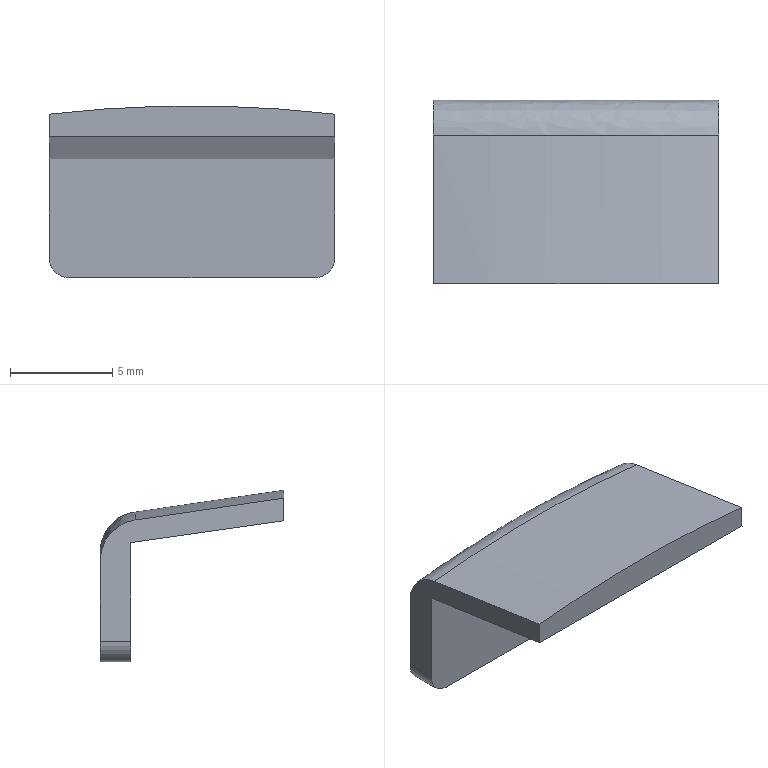Part | STEP file | ZXW735-L-95-05 | 1 solid | 15 faces | box 14 x 9 x 8.417 mm | volume 278.257 mm3 | plane 10 | cylinder 3 | other 1 | spline 1 | commonest cylinder face diameters 2 x2 61.422 x1
STEP:
#1=CARTESIAN_POINT('',(0.,0.,0.));
#2=DIRECTION('',(0.,0.,1.));
#3=DIRECTION('',(1.,0.,0.));
#4=AXIS2_PLACEMENT_3D('',#1,#2,#3);
#5=CARTESIAN_POINT('',(-23.763,12.127,8.554));
#6=VERTEX_POINT('',#5);
#7=CARTESIAN_POINT('',(-37.763,12.127,8.554));
#8=VERTEX_POINT('',#7);
#9=CARTESIAN_POINT('',(-24.693,12.127,8.661));
#10=CARTESIAN_POINT('',(-26.555,12.127,8.833));
#11=CARTESIAN_POINT('',(-29.36,12.127,8.962));
#12=CARTESIAN_POINT('',(-32.167,12.127,8.962));
#13=CARTESIAN_POINT('',(-34.971,12.127,8.833));
#14=CARTESIAN_POINT('',(-36.833,12.127,8.661));
#15=B_SPLINE_CURVE_WITH_KNOTS('',3,(#5,#9,#10,#11,#12,#13,#14,#7),.UNSPECIFIED.,.F.,.F.,(4,1,1,1,1,4),(0.,0.2,0.4,0.6,0.8,1.),.UNSPECIFIED.);
#16=EDGE_CURVE('',#6,#8,#15,.T.);
#17=ORIENTED_EDGE('',*,*,#16,.F.);
#18=CARTESIAN_POINT('',(-23.763,12.127,7.444));
#19=VERTEX_POINT('',#18);
#20=CARTESIAN_POINT('',(-23.763,12.127,7.444));
#21=DIRECTION('',(0.00001014,0.00001377,1.));
#22=VECTOR('',#21,1.11);
#23=LINE('',#20,#22);
#24=EDGE_CURVE('',#19,#6,#23,.T.);
#25=ORIENTED_EDGE('',*,*,#24,.F.);
#26=CARTESIAN_POINT('',(-37.763,12.127,7.444));
#27=VERTEX_POINT('',#26);
#28=CARTESIAN_POINT('',(-37.763,12.127,7.444));
#29=DIRECTION('',(1.,0.,0.000000407));
#30=VECTOR('',#29,14.);
#31=LINE('',#28,#30);
#32=EDGE_CURVE('',#27,#19,#31,.T.);
#33=ORIENTED_EDGE('',*,*,#32,.F.);
#34=CARTESIAN_POINT('',(-37.763,12.127,7.444));
#35=DIRECTION('',(-0.00001151,0.00000571,1.));
#36=VECTOR('',#35,1.11);
#37=LINE('',#34,#36);
#38=EDGE_CURVE('',#27,#8,#37,.T.);
#39=ORIENTED_EDGE('',*,*,#38,.T.);
#40=EDGE_LOOP('',(#17,#25,#33,#39));
#41=FACE_OUTER_BOUND('',#40,.F.);
#42=CARTESIAN_POINT('',(-37.363,12.127,5.74));
#43=DIRECTION('',(0.,1.,0.));
#44=DIRECTION('',(-1.,0.,-0.000000599));
#45=AXIS2_PLACEMENT_3D('',#42,#43,#44);
#46=PLANE('',#45);
#47=ADVANCED_FACE('',(#41),#46,.F.);
#48=CARTESIAN_POINT('',(-23.763,19.417,7.482));
#49=VERTEX_POINT('',#48);
#50=CARTESIAN_POINT('',(-23.763,19.417,7.482));
#51=DIRECTION('',(-0.000000599,-0.9894,0.1455));
#52=VECTOR('',#51,7.368);
#53=LINE('',#50,#52);
#54=EDGE_CURVE('',#49,#6,#53,.T.);
#55=ORIENTED_EDGE('',*,*,#54,.T.);
#56=ORIENTED_EDGE('',*,*,#16,.T.);
#57=CARTESIAN_POINT('',(-37.763,19.417,7.483));
#58=VERTEX_POINT('',#57);
#59=CARTESIAN_POINT('',(-37.763,12.127,8.554));
#60=DIRECTION('',(-0.000000416,0.9894,-0.1455));
#61=VECTOR('',#60,7.368);
#62=LINE('',#59,#61);
#63=EDGE_CURVE('',#8,#58,#62,.T.);
#64=ORIENTED_EDGE('',*,*,#63,.T.);
#65=CARTESIAN_POINT('',(-30.763,19.417,-53.205));
#66=DIRECTION('',(0.,1.,0.));
#67=DIRECTION('',(-0.1146,0.,0.9934));
#68=AXIS2_PLACEMENT_3D('',#65,#66,#67);
#69=CIRCLE('',#68,61.09);
#70=EDGE_CURVE('',#58,#49,#69,.T.);
#71=ORIENTED_EDGE('',*,*,#70,.T.);
#72=EDGE_LOOP('',(#55,#56,#64,#71));
#73=FACE_OUTER_BOUND('',#72,.F.);
#74=CARTESIAN_POINT('',(-30.763,10.927,-51.957));
#75=DIRECTION('',(0.,1.,0.));
#76=DIRECTION('',(-0.1277,0.,0.9918));
#77=AXIS2_PLACEMENT_3D('',#74,#75,#76);
#78=CIRCLE('',#77,61.09);
#79=TRIMMED_CURVE('',#78,(PARAMETER_VALUE(0.)),(PARAMETER_VALUE(14.671)),.T.,.UNSPECIFIED.);
#80=DIRECTION('',(0.00000009,0.9894,-0.1455));
#81=VECTOR('',#80,1.);
#82=SURFACE_OF_LINEAR_EXTRUSION('',#79,#81);
#83=ADVANCED_FACE('',(#73),#82,.T.);
#84=CARTESIAN_POINT('',(-23.763,21.127,1.54));
#85=VERTEX_POINT('',#84);
#86=CARTESIAN_POINT('',(-23.763,21.127,5.49));
#87=VERTEX_POINT('',#86);
#88=CARTESIAN_POINT('',(-23.763,21.127,1.54));
#89=DIRECTION('',(-0.000000635,0.,1.));
#90=VECTOR('',#89,3.95);
#91=LINE('',#88,#90);
#92=EDGE_CURVE('',#85,#87,#91,.T.);
#93=ORIENTED_EDGE('',*,*,#92,.F.);
#94=CARTESIAN_POINT('',(-23.763,19.627,1.54));
#95=VERTEX_POINT('',#94);
#96=CARTESIAN_POINT('',(-23.763,21.127,1.54));
#97=DIRECTION('',(-0.000000163,-1.,-0.000001718));
#98=VECTOR('',#97,1.5);
#99=LINE('',#96,#98);
#100=EDGE_CURVE('',#85,#95,#99,.T.);
#101=ORIENTED_EDGE('',*,*,#100,.T.);
#102=CARTESIAN_POINT('',(-23.763,19.627,6.374));
#103=VERTEX_POINT('',#102);
#104=CARTESIAN_POINT('',(-23.763,19.627,1.54));
#105=DIRECTION('',(-0.000000525,0.,1.));
#106=VECTOR('',#105,4.834);
#107=LINE('',#104,#106);
#108=EDGE_CURVE('',#95,#103,#107,.T.);
#109=ORIENTED_EDGE('',*,*,#108,.T.);
#110=CARTESIAN_POINT('',(-23.763,12.127,7.444));
#111=DIRECTION('',(0.000000107,0.99,-0.1412));
#112=VECTOR('',#111,7.576);
#113=LINE('',#110,#112);
#114=EDGE_CURVE('',#19,#103,#113,.T.);
#115=ORIENTED_EDGE('',*,*,#114,.F.);
#116=ORIENTED_EDGE('',*,*,#24,.T.);
#117=ORIENTED_EDGE('',*,*,#54,.F.);
#118=CARTESIAN_POINT('',(-23.763,19.417,7.482));
#119=CARTESIAN_POINT('',(-23.763,19.535,7.465));
#120=CARTESIAN_POINT('',(-23.763,19.764,7.41));
#121=CARTESIAN_POINT('',(-23.763,20.093,7.265));
#122=CARTESIAN_POINT('',(-23.763,20.39,7.065));
#123=CARTESIAN_POINT('',(-23.763,20.647,6.816));
#124=CARTESIAN_POINT('',(-23.763,20.856,6.524));
#125=CARTESIAN_POINT('',(-23.763,21.01,6.199));
#126=CARTESIAN_POINT('',(-23.763,21.106,5.851));
#127=CARTESIAN_POINT('',(-23.763,21.127,5.612));
#128=CARTESIAN_POINT('',(-23.763,21.127,5.49));
#129=B_SPLINE_CURVE_WITH_KNOTS('',3,(#118,#119,#120,#121,#122,#123,#124,#125,#126,#127,#128),.UNSPECIFIED.,.F.,.F.,(4,1,1,1,1,1,1,1,4),(0.,0.125,0.25,0.375,0.5,0.625,0.75,0.875,1.),.UNSPECIFIED.);
#130=EDGE_CURVE('',#49,#87,#129,.T.);
#131=ORIENTED_EDGE('',*,*,#130,.T.);
#132=EDGE_LOOP('',(#93,#101,#109,#115,#116,#117,#131));
#133=FACE_OUTER_BOUND('',#132,.F.);
#134=CARTESIAN_POINT('',(-23.763,27.279,-9.26));
#135=DIRECTION('',(1.,0.,0.000000621));
#136=DIRECTION('',(-0.000000621,0.,1.));
#137=AXIS2_PLACEMENT_3D('',#134,#135,#136);
#138=PLANE('',#137);
#139=ADVANCED_FACE('',(#133),#138,.T.);
#140=CARTESIAN_POINT('',(-37.763,21.127,1.54));
#141=VERTEX_POINT('',#140);
#142=CARTESIAN_POINT('',(-37.763,21.127,5.49));
#143=VERTEX_POINT('',#142);
#144=CARTESIAN_POINT('',(-37.763,21.127,1.54));
#145=DIRECTION('',(-0.000000625,0.,1.));
#146=VECTOR('',#145,3.95);
#147=LINE('',#144,#146);
#148=EDGE_CURVE('',#141,#143,#147,.T.);
#149=ORIENTED_EDGE('',*,*,#148,.F.);
#150=CARTESIAN_POINT('',(-36.763,21.127,0.5396));
#151=VERTEX_POINT('',#150);
#152=CARTESIAN_POINT('',(-36.763,21.127,1.54));
#153=DIRECTION('',(0.,1.,0.));
#154=DIRECTION('',(0.0000187,0.,-1.));
#155=AXIS2_PLACEMENT_3D('',#152,#153,#154);
#156=CIRCLE('',#155,1.);
#157=EDGE_CURVE('',#151,#141,#156,.T.);
#158=ORIENTED_EDGE('',*,*,#157,.F.);
#159=CARTESIAN_POINT('',(-24.763,21.127,0.5396));
#160=VERTEX_POINT('',#159);
#161=CARTESIAN_POINT('',(-24.763,21.127,0.5396));
#162=DIRECTION('',(-1.,0.,-0.000000397));
#163=VECTOR('',#162,12.);
#164=LINE('',#161,#163);
#165=EDGE_CURVE('',#160,#151,#164,.T.);
#166=ORIENTED_EDGE('',*,*,#165,.F.);
#167=CARTESIAN_POINT('',(-24.763,21.127,1.54));
#168=DIRECTION('',(0.,1.,0.));
#169=DIRECTION('',(1.,0.,-0.000000136));
#170=AXIS2_PLACEMENT_3D('',#167,#168,#169);
#171=CIRCLE('',#170,1.);
#172=EDGE_CURVE('',#85,#160,#171,.T.);
#173=ORIENTED_EDGE('',*,*,#172,.F.);
#174=ORIENTED_EDGE('',*,*,#92,.T.);
#175=CARTESIAN_POINT('',(-37.763,21.127,5.49));
#176=CARTESIAN_POINT('',(-33.119,21.127,6.042));
#177=CARTESIAN_POINT('',(-28.411,21.127,6.042));
#178=CARTESIAN_POINT('',(-23.763,21.127,5.49));
#179=B_SPLINE_CURVE_WITH_KNOTS('',3,(#175,#176,#177,#178),.UNSPECIFIED.,.F.,.F.,(4,4),(0.,1.),.UNSPECIFIED.);
#180=EDGE_CURVE('',#143,#87,#179,.T.);
#181=ORIENTED_EDGE('',*,*,#180,.F.);
#182=EDGE_LOOP('',(#149,#158,#166,#173,#174,#181));
#183=FACE_OUTER_BOUND('',#182,.F.);
#184=CARTESIAN_POINT('',(-36.62,21.127,5.114));
#185=VERTEX_POINT('',#184);
#186=CARTESIAN_POINT('',(-30.763,21.127,1.576));
#187=VERTEX_POINT('',#186);
#188=CARTESIAN_POINT('',(-36.62,21.127,5.114));
#189=DIRECTION('',(0.856,0.,-0.517));
#190=VECTOR('',#189,6.842);
#191=LINE('',#188,#190);
#192=EDGE_CURVE('',#185,#187,#191,.T.);
#193=ORIENTED_EDGE('',*,*,#192,.F.);
#194=CARTESIAN_POINT('',(-24.898,21.127,5.118));
#195=VERTEX_POINT('',#194);
#196=CARTESIAN_POINT('',(-30.772,21.127,35.262));
#197=DIRECTION('',(0.,1.,0.));
#198=DIRECTION('',(0.1912,0.,-0.9815));
#199=AXIS2_PLACEMENT_3D('',#196,#197,#198);
#200=CIRCLE('',#199,30.711);
#201=EDGE_CURVE('',#195,#185,#200,.T.);
#202=ORIENTED_EDGE('',*,*,#201,.F.);
#203=CARTESIAN_POINT('',(-30.763,21.127,1.576));
#204=DIRECTION('',(0.856,0.,0.517));
#205=VECTOR('',#204,6.852);
#206=LINE('',#203,#205);
#207=EDGE_CURVE('',#187,#195,#206,.T.);
#208=ORIENTED_EDGE('',*,*,#207,.F.);
#209=EDGE_LOOP('',(#193,#202,#208));
#210=FACE_BOUND('',#209,.F.);
#211=CARTESIAN_POINT('',(-38.363,21.127,5.74));
#212=DIRECTION('',(0.,1.,0.));
#213=DIRECTION('',(-1.,0.,-0.000000599));
#214=AXIS2_PLACEMENT_3D('',#211,#212,#213);
#215=PLANE('',#214);
#216=ADVANCED_FACE('',(#183,#210),#215,.T.);
#217=CARTESIAN_POINT('',(-30.763,20.877,1.576));
#218=VERTEX_POINT('',#217);
#219=CARTESIAN_POINT('',(-30.763,21.127,1.576));
#220=DIRECTION('',(0.,-1.,0.));
#221=VECTOR('',#220,0.25);
#222=LINE('',#219,#221);
#223=EDGE_CURVE('',#187,#218,#222,.T.);
#224=ORIENTED_EDGE('',*,*,#223,.T.);
#225=CARTESIAN_POINT('',(-36.62,20.877,5.114));
#226=VERTEX_POINT('',#225);
#227=CARTESIAN_POINT('',(-30.763,20.877,1.576));
#228=DIRECTION('',(-0.856,0.,0.517));
#229=VECTOR('',#228,6.842);
#230=LINE('',#227,#229);
#231=EDGE_CURVE('',#218,#226,#230,.T.);
#232=ORIENTED_EDGE('',*,*,#231,.T.);
#233=CARTESIAN_POINT('',(-36.62,20.877,5.114));
#234=DIRECTION('',(0.,1.,0.));
#235=VECTOR('',#234,0.25);
#236=LINE('',#233,#235);
#237=EDGE_CURVE('',#226,#185,#236,.T.);
#238=ORIENTED_EDGE('',*,*,#237,.T.);
#239=ORIENTED_EDGE('',*,*,#192,.T.);
#240=EDGE_LOOP('',(#224,#232,#238,#239));
#241=FACE_OUTER_BOUND('',#240,.F.);
#242=CARTESIAN_POINT('',(-36.731,20.627,5.181));
#243=DIRECTION('',(0.517,0.,0.856));
#244=DIRECTION('',(-0.856,0.,0.517));
#245=AXIS2_PLACEMENT_3D('',#242,#243,#244);
#246=PLANE('',#245);
#247=ADVANCED_FACE('',(#241),#246,.T.);
#248=CARTESIAN_POINT('',(-24.898,20.877,5.118));
#249=VERTEX_POINT('',#248);
#250=CARTESIAN_POINT('',(-24.898,21.127,5.118));
#251=DIRECTION('',(0.,-1.,0.));
#252=VECTOR('',#251,0.25);
#253=LINE('',#250,#252);
#254=EDGE_CURVE('',#195,#249,#253,.T.);
#255=ORIENTED_EDGE('',*,*,#254,.T.);
#256=CARTESIAN_POINT('',(-24.898,20.877,5.118));
#257=DIRECTION('',(-0.856,0.,-0.517));
#258=VECTOR('',#257,6.852);
#259=LINE('',#256,#258);
#260=EDGE_CURVE('',#249,#218,#259,.T.);
#261=ORIENTED_EDGE('',*,*,#260,.T.);
#262=ORIENTED_EDGE('',*,*,#223,.F.);
#263=ORIENTED_EDGE('',*,*,#207,.T.);
#264=EDGE_LOOP('',(#255,#261,#262,#263));
#265=FACE_OUTER_BOUND('',#264,.F.);
#266=CARTESIAN_POINT('',(-30.626,20.627,1.659));
#267=DIRECTION('',(-0.517,0.,0.856));
#268=DIRECTION('',(-0.856,0.,-0.517));
#269=AXIS2_PLACEMENT_3D('',#266,#267,#268);
#270=PLANE('',#269);
#271=ADVANCED_FACE('',(#265),#270,.T.);
#272=ORIENTED_EDGE('',*,*,#237,.F.);
#273=CARTESIAN_POINT('',(-30.772,20.877,35.262));
#274=DIRECTION('',(0.,-1.,0.));
#275=DIRECTION('',(-0.1904,0.,-0.9817));
#276=AXIS2_PLACEMENT_3D('',#273,#274,#275);
#277=CIRCLE('',#276,30.711);
#278=EDGE_CURVE('',#226,#249,#277,.T.);
#279=ORIENTED_EDGE('',*,*,#278,.T.);
#280=ORIENTED_EDGE('',*,*,#254,.F.);
#281=ORIENTED_EDGE('',*,*,#201,.T.);
#282=EDGE_LOOP('',(#272,#279,#280,#281));
#283=FACE_OUTER_BOUND('',#282,.F.);
#284=CARTESIAN_POINT('',(-30.772,21.002,35.262));
#285=DIRECTION('',(0.,1.,0.));
#286=DIRECTION('',(0.1912,0.,-0.9815));
#287=AXIS2_PLACEMENT_3D('',#284,#285,#286);
#288=CYLINDRICAL_SURFACE('',#287,30.711);
#289=ADVANCED_FACE('',(#283),#288,.T.);
#290=ORIENTED_EDGE('',*,*,#278,.F.);
#291=ORIENTED_EDGE('',*,*,#231,.F.);
#292=ORIENTED_EDGE('',*,*,#260,.F.);
#293=EDGE_LOOP('',(#290,#291,#292));
#294=FACE_OUTER_BOUND('',#293,.F.);
#295=CARTESIAN_POINT('',(-38.363,20.877,6.34));
#296=DIRECTION('',(0.,1.,0.));
#297=DIRECTION('',(-1.,0.,-0.000000599));
#298=AXIS2_PLACEMENT_3D('',#295,#296,#297);
#299=PLANE('',#298);
#300=ADVANCED_FACE('',(#294),#299,.T.);
#301=ORIENTED_EDGE('',*,*,#63,.F.);
#302=ORIENTED_EDGE('',*,*,#38,.F.);
#303=CARTESIAN_POINT('',(-37.763,19.627,6.374));
#304=VERTEX_POINT('',#303);
#305=CARTESIAN_POINT('',(-37.763,19.627,6.374));
#306=DIRECTION('',(-0.000000118,-0.99,0.1412));
#307=VECTOR('',#306,7.576);
#308=LINE('',#305,#307);
#309=EDGE_CURVE('',#304,#27,#308,.T.);
#310=ORIENTED_EDGE('',*,*,#309,.F.);
#311=CARTESIAN_POINT('',(-37.763,19.627,1.54));
#312=VERTEX_POINT('',#311);
#313=CARTESIAN_POINT('',(-37.763,19.627,1.54));
#314=DIRECTION('',(-0.000000561,0.,1.));
#315=VECTOR('',#314,4.834);
#316=LINE('',#313,#315);
#317=EDGE_CURVE('',#312,#304,#316,.T.);
#318=ORIENTED_EDGE('',*,*,#317,.F.);
#319=CARTESIAN_POINT('',(-37.763,19.627,1.54));
#320=DIRECTION('',(0.000000168,1.,-0.000001743));
#321=VECTOR('',#320,1.5);
#322=LINE('',#319,#321);
#323=EDGE_CURVE('',#312,#141,#322,.T.);
#324=ORIENTED_EDGE('',*,*,#323,.T.);
#325=ORIENTED_EDGE('',*,*,#148,.T.);
#326=CARTESIAN_POINT('',(-37.763,21.127,5.611));
#327=CARTESIAN_POINT('',(-37.763,21.106,5.85));
#328=CARTESIAN_POINT('',(-37.763,21.01,6.2));
#329=CARTESIAN_POINT('',(-37.763,20.855,6.525));
#330=CARTESIAN_POINT('',(-37.763,20.646,6.816));
#331=CARTESIAN_POINT('',(-37.763,20.389,7.066));
#332=CARTESIAN_POINT('',(-37.763,20.093,7.265));
#333=CARTESIAN_POINT('',(-37.763,19.765,7.41));
#334=CARTESIAN_POINT('',(-37.763,19.535,7.465));
#335=CARTESIAN_POINT('',(-37.763,19.417,7.482));
#336=B_SPLINE_CURVE_WITH_KNOTS('',3,(#142,#326,#327,#328,#329,#330,#331,#332,#333,#334,#335),.UNSPECIFIED.,.F.,.F.,(4,1,1,1,1,1,1,1,4),(0.,0.125,0.25,0.375,0.5,0.625,0.75,0.875,1.),.UNSPECIFIED.);
#337=EDGE_CURVE('',#143,#58,#336,.T.);
#338=ORIENTED_EDGE('',*,*,#337,.T.);
#339=EDGE_LOOP('',(#301,#302,#310,#318,#324,#325,#338));
#340=FACE_OUTER_BOUND('',#339,.F.);
#341=CARTESIAN_POINT('',(-37.763,27.279,0.7396));
#342=DIRECTION('',(-1.,0.,-0.000000671));
#343=DIRECTION('',(0.000000671,0.,-1.));
#344=AXIS2_PLACEMENT_3D('',#341,#342,#343);
#345=PLANE('',#344);
#346=ADVANCED_FACE('',(#340),#345,.T.);
#347=ORIENTED_EDGE('',*,*,#32,.T.);
#348=ORIENTED_EDGE('',*,*,#114,.T.);
#349=CARTESIAN_POINT('',(-37.763,19.627,6.374));
#350=DIRECTION('',(1.,0.,0.000000307));
#351=VECTOR('',#350,14.);
#352=LINE('',#349,#351);
#353=EDGE_CURVE('',#304,#103,#352,.T.);
#354=ORIENTED_EDGE('',*,*,#353,.F.);
#355=ORIENTED_EDGE('',*,*,#309,.T.);
#356=EDGE_LOOP('',(#347,#348,#354,#355));
#357=FACE_OUTER_BOUND('',#356,.F.);
#358=CARTESIAN_POINT('',(22.837,20.794,6.208));
#359=DIRECTION('',(0.000000296,-0.1412,-0.99));
#360=DIRECTION('',(0.000000042,0.99,-0.1412));
#361=AXIS2_PLACEMENT_3D('',#358,#359,#360);
#362=PLANE('',#361);
#363=ADVANCED_FACE('',(#357),#362,.T.);
#364=ORIENTED_EDGE('',*,*,#317,.T.);
#365=ORIENTED_EDGE('',*,*,#353,.T.);
#366=ORIENTED_EDGE('',*,*,#108,.F.);
#367=CARTESIAN_POINT('',(-24.763,19.627,0.5396));
#368=VERTEX_POINT('',#367);
#369=CARTESIAN_POINT('',(-24.763,19.627,1.54));
#370=DIRECTION('',(0.,-1.,0.));
#371=DIRECTION('',(0.000000494,0.,-1.));
#372=AXIS2_PLACEMENT_3D('',#369,#370,#371);
#373=CIRCLE('',#372,1.);
#374=EDGE_CURVE('',#368,#95,#373,.T.);
#375=ORIENTED_EDGE('',*,*,#374,.F.);
#376=CARTESIAN_POINT('',(-36.763,19.627,0.5396));
#377=VERTEX_POINT('',#376);
#378=CARTESIAN_POINT('',(-36.763,19.627,0.5396));
#379=DIRECTION('',(1.,0.,0.000000297));
#380=VECTOR('',#379,12.);
#381=LINE('',#378,#380);
#382=EDGE_CURVE('',#377,#368,#381,.T.);
#383=ORIENTED_EDGE('',*,*,#382,.F.);
#384=CARTESIAN_POINT('',(-36.763,19.627,1.54));
#385=DIRECTION('',(0.,-1.,0.));
#386=DIRECTION('',(-1.,0.,0.000008611));
#387=AXIS2_PLACEMENT_3D('',#384,#385,#386);
#388=CIRCLE('',#387,1.);
#389=EDGE_CURVE('',#312,#377,#388,.T.);
#390=ORIENTED_EDGE('',*,*,#389,.F.);
#391=EDGE_LOOP('',(#364,#365,#366,#375,#383,#390));
#392=FACE_OUTER_BOUND('',#391,.F.);
#393=CARTESIAN_POINT('',(-38.763,19.627,7.383));
#394=DIRECTION('',(0.,-1.,0.));
#395=DIRECTION('',(1.,0.,0.0000003));
#396=AXIS2_PLACEMENT_3D('',#393,#394,#395);
#397=PLANE('',#396);
#398=ADVANCED_FACE('',(#392),#397,.T.);
#399=CARTESIAN_POINT('',(-24.763,19.627,0.5396));
#400=DIRECTION('',(0.000004046,1.,0.000000399));
#401=VECTOR('',#400,1.5);
#402=LINE('',#399,#401);
#403=EDGE_CURVE('',#368,#160,#402,.T.);
#404=ORIENTED_EDGE('',*,*,#403,.F.);
#405=ORIENTED_EDGE('',*,*,#374,.T.);
#406=ORIENTED_EDGE('',*,*,#100,.F.);
#407=ORIENTED_EDGE('',*,*,#172,.T.);
#408=EDGE_LOOP('',(#404,#405,#406,#407));
#409=FACE_OUTER_BOUND('',#408,.F.);
#410=CARTESIAN_POINT('',(-24.763,19.382,1.54));
#411=DIRECTION('',(0.,-1.,0.));
#412=DIRECTION('',(0.000000299,0.,-1.));
#413=AXIS2_PLACEMENT_3D('',#410,#411,#412);
#414=CYLINDRICAL_SURFACE('',#413,1.);
#415=ADVANCED_FACE('',(#409),#414,.T.);
#416=CARTESIAN_POINT('',(-36.763,21.127,0.5396));
#417=DIRECTION('',(-0.000004046,-1.,0.000000399));
#418=VECTOR('',#417,1.5);
#419=LINE('',#416,#418);
#420=EDGE_CURVE('',#151,#377,#419,.T.);
#421=ORIENTED_EDGE('',*,*,#420,.T.);
#422=ORIENTED_EDGE('',*,*,#382,.T.);
#423=ORIENTED_EDGE('',*,*,#403,.T.);
#424=ORIENTED_EDGE('',*,*,#165,.T.);
#425=EDGE_LOOP('',(#421,#422,#423,#424));
#426=FACE_OUTER_BOUND('',#425,.F.);
#427=CARTESIAN_POINT('',(-38.763,19.382,0.5396));
#428=DIRECTION('',(0.000000296,0.,-1.));
#429=DIRECTION('',(0.,1.,0.));
#430=AXIS2_PLACEMENT_3D('',#427,#428,#429);
#431=PLANE('',#430);
#432=ADVANCED_FACE('',(#426),#431,.T.);
#433=ORIENTED_EDGE('',*,*,#323,.F.);
#434=ORIENTED_EDGE('',*,*,#389,.T.);
#435=ORIENTED_EDGE('',*,*,#420,.F.);
#436=ORIENTED_EDGE('',*,*,#157,.T.);
#437=EDGE_LOOP('',(#433,#434,#435,#436));
#438=FACE_OUTER_BOUND('',#437,.F.);
#439=CARTESIAN_POINT('',(-36.763,27.279,1.54));
#440=DIRECTION('',(0.,-1.,0.));
#441=DIRECTION('',(0.000000299,0.,-1.));
#442=AXIS2_PLACEMENT_3D('',#439,#440,#441);
#443=CYLINDRICAL_SURFACE('',#442,1.);
#444=ADVANCED_FACE('',(#438),#443,.T.);
#445=ORIENTED_EDGE('',*,*,#130,.F.);
#446=ORIENTED_EDGE('',*,*,#70,.F.);
#447=ORIENTED_EDGE('',*,*,#337,.F.);
#448=ORIENTED_EDGE('',*,*,#180,.T.);
#449=EDGE_LOOP('',(#445,#446,#447,#448));
#450=FACE_OUTER_BOUND('',#449,.F.);
#451=CARTESIAN_POINT('',(-38.141,19.387,7.442));
#452=CARTESIAN_POINT('',(-38.125,20.444,7.304));
#453=CARTESIAN_POINT('',(-38.027,21.142,6.504));
#454=CARTESIAN_POINT('',(-37.899,21.127,5.445));
#455=CARTESIAN_POINT('',(-33.249,19.389,8.035));
#456=CARTESIAN_POINT('',(-33.245,20.446,7.895));
#457=CARTESIAN_POINT('',(-33.212,21.142,7.087));
#458=CARTESIAN_POINT('',(-33.165,21.127,6.019));
#459=CARTESIAN_POINT('',(-28.281,19.389,8.035));
#460=CARTESIAN_POINT('',(-28.285,20.446,7.895));
#461=CARTESIAN_POINT('',(-28.319,21.142,7.087));
#462=CARTESIAN_POINT('',(-28.365,21.127,6.02));
#463=CARTESIAN_POINT('',(-23.385,19.387,7.442));
#464=CARTESIAN_POINT('',(-23.402,20.444,7.304));
#465=CARTESIAN_POINT('',(-23.499,21.142,6.504));
#466=CARTESIAN_POINT('',(-23.627,21.127,5.445));
#467=(BOUNDED_SURFACE()B_SPLINE_SURFACE(3,3,((#451,#452,#453,#454),(#455,#456,#457,#458),(#459,#460,#461,#462),(#463,#464,#465,#466)),.UNSPECIFIED.,.F.,.F.,.F.)B_SPLINE_SURFACE_WITH_KNOTS((4,4),(4,4),(-0.003948,1.004),(-0.01137,1.011),.UNSPECIFIED.)GEOMETRIC_REPRESENTATION_ITEM()RATIONAL_B_SPLINE_SURFACE(((1.006,0.8359,0.8358,1.005),(1.006,0.8362,0.8361,1.005),(1.006,0.8362,0.8361,1.005),(1.006,0.8359,0.8358,1.005)))REPRESENTATION_ITEM('')SURFACE());
#468=ADVANCED_FACE('',(#450),#467,.T.);
#469=CLOSED_SHELL('',(#47,#83,#139,#216,#247,#271,#289,#300,#346,#363,#398,#415,#432,#444,#468));
#470=MANIFOLD_SOLID_BREP('',#469);
#471=(LENGTH_UNIT()NAMED_UNIT(*)SI_UNIT(.MILLI.,.METRE.));
#472=UNCERTAINTY_MEASURE_WITH_UNIT(LENGTH_MEASURE(0.001905),#471,'','');
#473=(NAMED_UNIT(*)PLANE_ANGLE_UNIT()SI_UNIT($,.RADIAN.));
#474=PLANE_ANGLE_MEASURE_WITH_UNIT(PLANE_ANGLE_MEASURE(0.01745),#473);
#475=(CONVERSION_BASED_UNIT('DEGREE',#474)NAMED_UNIT(*)PLANE_ANGLE_UNIT());
#476=(NAMED_UNIT(*)SI_UNIT($,.STERADIAN.)SOLID_ANGLE_UNIT());
#477=(GEOMETRIC_REPRESENTATION_CONTEXT(3)GLOBAL_UNCERTAINTY_ASSIGNED_CONTEXT((#472))GLOBAL_UNIT_ASSIGNED_CONTEXT((#471,#475,#476))REPRESENTATION_CONTEXT('',''));
#478=ADVANCED_BREP_SHAPE_REPRESENTATION('',(#4,#470),#477);